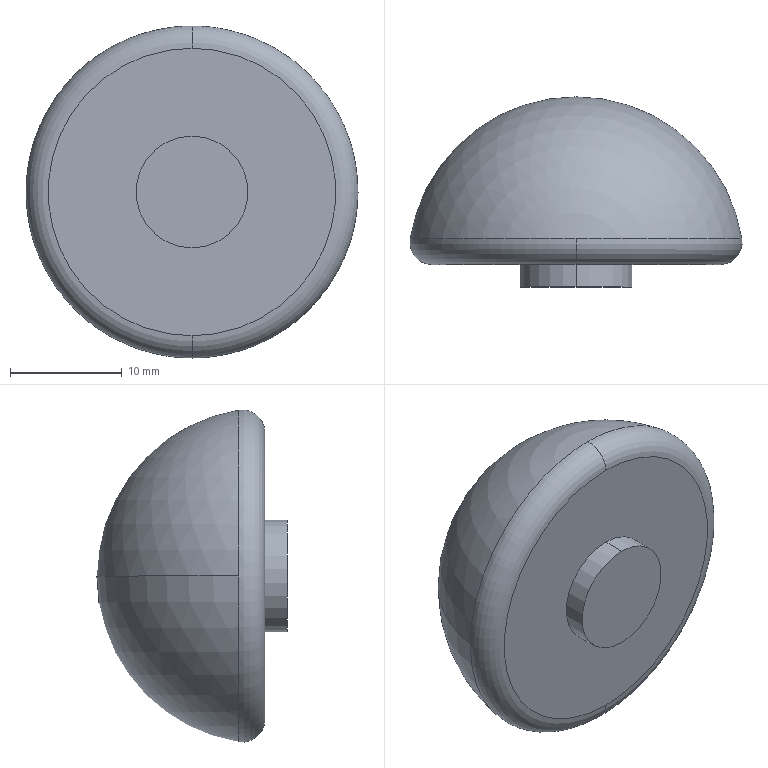Part | SolidWorks | features Fillet 1, ICE 1, Revolution 1 | 1 solid | 8 faces | box 29.69 x 17 x 29.69 mm | volume 7127 mm3 | torus 2 | cylinder 2 | sphere 2 | plane 2 | commonest cylinder face diameters 10 x2
STEP:
#1=CARTESIAN_POINT('',(0.,2.308,14.821));
#2=VERTEX_POINT('',#1);
#3=CARTESIAN_POINT('',(14.821,2.308,0.));
#4=VERTEX_POINT('',#3);
#5=CARTESIAN_POINT('',(0.,2.308,0.));
#6=DIRECTION('',(0.,1.,0.));
#7=DIRECTION('',(0.,0.,-1.));
#8=AXIS2_PLACEMENT_3D('',#5,#6,#7);
#9=CIRCLE('',#8,14.821);
#10=EDGE_CURVE('',#2,#4,#9,.T.);
#11=ORIENTED_EDGE('',*,*,#10,.F.);
#12=CARTESIAN_POINT('',(0.,0.,12.845));
#13=VERTEX_POINT('',#12);
#14=CARTESIAN_POINT('',(0.,2.,12.845));
#15=DIRECTION('',(1.,0.,0.));
#16=DIRECTION('',(0.,0.,-1.));
#17=AXIS2_PLACEMENT_3D('',#14,#15,#16);
#18=CIRCLE('',#17,2.);
#19=EDGE_CURVE('',#2,#13,#18,.T.);
#20=ORIENTED_EDGE('',*,*,#19,.T.);
#21=CARTESIAN_POINT('',(0.,0.,-12.845));
#22=VERTEX_POINT('',#21);
#23=CARTESIAN_POINT('',(0.,0.,0.));
#24=DIRECTION('',(0.,-1.,0.));
#25=DIRECTION('',(0.,0.,-1.));
#26=AXIS2_PLACEMENT_3D('',#23,#24,#25);
#27=CIRCLE('',#26,12.845);
#28=EDGE_CURVE('',#22,#13,#27,.T.);
#29=ORIENTED_EDGE('',*,*,#28,.F.);
#30=CARTESIAN_POINT('',(0.,2.308,-14.821));
#31=VERTEX_POINT('',#30);
#32=CARTESIAN_POINT('',(0.,2.,-12.845));
#33=DIRECTION('',(-1.,0.,0.));
#34=DIRECTION('',(0.,0.,1.));
#35=AXIS2_PLACEMENT_3D('',#32,#33,#34);
#36=CIRCLE('',#35,2.);
#37=EDGE_CURVE('',#31,#22,#36,.T.);
#38=ORIENTED_EDGE('',*,*,#37,.F.);
#39=CARTESIAN_POINT('',(0.,2.308,0.));
#40=DIRECTION('',(0.,1.,0.));
#41=DIRECTION('',(0.,0.,-1.));
#42=AXIS2_PLACEMENT_3D('',#39,#40,#41);
#43=CIRCLE('',#42,14.821);
#44=EDGE_CURVE('',#4,#31,#43,.T.);
#45=ORIENTED_EDGE('',*,*,#44,.F.);
#46=EDGE_LOOP('',(#11,#20,#29,#38,#45));
#47=FACE_OUTER_BOUND('',#46,.T.);
#48=CARTESIAN_POINT('',(0.,2.,0.));
#49=DIRECTION('',(0.,-1.,0.));
#50=DIRECTION('',(0.,0.,-1.));
#51=AXIS2_PLACEMENT_3D('',#48,#49,#50);
#52=TOROIDAL_SURFACE('',#51,12.845,2.);
#53=ADVANCED_FACE('',(#47),#52,.T.);
#54=CARTESIAN_POINT('',(0.,-2.,-5.));
#55=VERTEX_POINT('',#54);
#56=CARTESIAN_POINT('',(0.,-2.,5.));
#57=VERTEX_POINT('',#56);
#58=CARTESIAN_POINT('',(0.,-2.,0.));
#59=DIRECTION('',(0.,-1.,0.));
#60=DIRECTION('',(0.,0.,-1.));
#61=AXIS2_PLACEMENT_3D('',#58,#59,#60);
#62=CIRCLE('',#61,5.);
#63=EDGE_CURVE('',#55,#57,#62,.T.);
#64=ORIENTED_EDGE('',*,*,#63,.F.);
#65=CARTESIAN_POINT('',(0.,0.,-5.));
#66=VERTEX_POINT('',#65);
#67=CARTESIAN_POINT('',(0.,-2.,-5.));
#68=DIRECTION('',(0.,1.,0.));
#69=VECTOR('',#68,1000.);
#70=LINE('',#67,#69);
#71=EDGE_CURVE('',#55,#66,#70,.T.);
#72=ORIENTED_EDGE('',*,*,#71,.T.);
#73=CARTESIAN_POINT('',(0.,0.,5.));
#74=VERTEX_POINT('',#73);
#75=CARTESIAN_POINT('',(0.,0.,0.));
#76=DIRECTION('',(0.,-1.,0.));
#77=DIRECTION('',(0.,0.,-1.));
#78=AXIS2_PLACEMENT_3D('',#75,#76,#77);
#79=CIRCLE('',#78,5.);
#80=EDGE_CURVE('',#66,#74,#79,.T.);
#81=ORIENTED_EDGE('',*,*,#80,.T.);
#82=CARTESIAN_POINT('',(0.,-2.,5.));
#83=DIRECTION('',(0.,1.,0.));
#84=VECTOR('',#83,1000.);
#85=LINE('',#82,#84);
#86=EDGE_CURVE('',#57,#74,#85,.T.);
#87=ORIENTED_EDGE('',*,*,#86,.F.);
#88=EDGE_LOOP('',(#64,#72,#81,#87));
#89=FACE_OUTER_BOUND('',#88,.T.);
#90=CARTESIAN_POINT('',(0.,-2.,0.));
#91=DIRECTION('',(0.,1.,0.));
#92=DIRECTION('',(0.,0.,1.));
#93=AXIS2_PLACEMENT_3D('',#90,#91,#92);
#94=CYLINDRICAL_SURFACE('',#93,5.);
#95=ADVANCED_FACE('',(#89),#94,.T.);
#96=CARTESIAN_POINT('',(0.,15.,0.));
#97=VERTEX_POINT('',#96);
#98=CARTESIAN_POINT('',(0.,0.,0.));
#99=DIRECTION('',(0.,0.,-1.));
#100=DIRECTION('',(-1.,0.,0.));
#101=AXIS2_PLACEMENT_3D('',#98,#99,#100);
#102=CIRCLE('',#101,15.);
#103=EDGE_CURVE('',#97,#4,#102,.T.);
#104=ORIENTED_EDGE('',*,*,#103,.F.);
#105=CARTESIAN_POINT('',(-14.821,2.308,0.));
#106=VERTEX_POINT('',#105);
#107=CARTESIAN_POINT('',(0.,0.,0.));
#108=DIRECTION('',(0.,0.,1.));
#109=DIRECTION('',(1.,0.,0.));
#110=AXIS2_PLACEMENT_3D('',#107,#108,#109);
#111=CIRCLE('',#110,15.);
#112=EDGE_CURVE('',#97,#106,#111,.T.);
#113=ORIENTED_EDGE('',*,*,#112,.T.);
#114=CARTESIAN_POINT('',(0.,2.308,0.));
#115=DIRECTION('',(0.,1.,0.));
#116=DIRECTION('',(0.,0.,-1.));
#117=AXIS2_PLACEMENT_3D('',#114,#115,#116);
#118=CIRCLE('',#117,14.821);
#119=EDGE_CURVE('',#106,#2,#118,.T.);
#120=ORIENTED_EDGE('',*,*,#119,.T.);
#121=ORIENTED_EDGE('',*,*,#10,.T.);
#122=EDGE_LOOP('',(#104,#113,#120,#121));
#123=FACE_OUTER_BOUND('',#122,.T.);
#124=CARTESIAN_POINT('',(0.,0.,0.));
#125=DIRECTION('',(0.,0.,1.));
#126=DIRECTION('',(1.,0.,0.));
#127=AXIS2_PLACEMENT_3D('',#124,#125,#126);
#128=SPHERICAL_SURFACE('',#127,15.);
#129=ADVANCED_FACE('',(#123),#128,.T.);
#130=ORIENTED_EDGE('',*,*,#28,.T.);
#131=CARTESIAN_POINT('',(0.,0.,0.));
#132=DIRECTION('',(0.,-1.,0.));
#133=DIRECTION('',(0.,0.,-1.));
#134=AXIS2_PLACEMENT_3D('',#131,#132,#133);
#135=CIRCLE('',#134,12.845);
#136=EDGE_CURVE('',#13,#22,#135,.T.);
#137=ORIENTED_EDGE('',*,*,#136,.T.);
#138=EDGE_LOOP('',(#130,#137));
#139=FACE_OUTER_BOUND('',#138,.T.);
#140=CARTESIAN_POINT('',(0.,0.,0.));
#141=DIRECTION('',(0.,-1.,0.));
#142=DIRECTION('',(0.,0.,-1.));
#143=AXIS2_PLACEMENT_3D('',#140,#141,#142);
#144=CIRCLE('',#143,5.);
#145=EDGE_CURVE('',#74,#66,#144,.T.);
#146=ORIENTED_EDGE('',*,*,#145,.F.);
#147=ORIENTED_EDGE('',*,*,#80,.F.);
#148=EDGE_LOOP('',(#146,#147));
#149=FACE_BOUND('',#148,.T.);
#150=CARTESIAN_POINT('',(0.,0.,0.));
#151=DIRECTION('',(0.,-1.,0.));
#152=DIRECTION('',(0.,0.,-1.));
#153=AXIS2_PLACEMENT_3D('',#150,#151,#152);
#154=PLANE('',#153);
#155=ADVANCED_FACE('',(#139,#149),#154,.T.);
#156=ORIENTED_EDGE('',*,*,#112,.F.);
#157=ORIENTED_EDGE('',*,*,#103,.T.);
#158=ORIENTED_EDGE('',*,*,#44,.T.);
#159=CARTESIAN_POINT('',(0.,2.308,0.));
#160=DIRECTION('',(0.,1.,0.));
#161=DIRECTION('',(0.,0.,-1.));
#162=AXIS2_PLACEMENT_3D('',#159,#160,#161);
#163=CIRCLE('',#162,14.821);
#164=EDGE_CURVE('',#31,#106,#163,.T.);
#165=ORIENTED_EDGE('',*,*,#164,.T.);
#166=EDGE_LOOP('',(#156,#157,#158,#165));
#167=FACE_OUTER_BOUND('',#166,.T.);
#168=CARTESIAN_POINT('',(0.,0.,0.));
#169=DIRECTION('',(0.,0.,1.));
#170=DIRECTION('',(1.,0.,0.));
#171=AXIS2_PLACEMENT_3D('',#168,#169,#170);
#172=SPHERICAL_SURFACE('',#171,15.);
#173=ADVANCED_FACE('',(#167),#172,.T.);
#174=ORIENTED_EDGE('',*,*,#71,.F.);
#175=CARTESIAN_POINT('',(0.,-2.,0.));
#176=DIRECTION('',(0.,-1.,0.));
#177=DIRECTION('',(0.,0.,-1.));
#178=AXIS2_PLACEMENT_3D('',#175,#176,#177);
#179=CIRCLE('',#178,5.);
#180=EDGE_CURVE('',#57,#55,#179,.T.);
#181=ORIENTED_EDGE('',*,*,#180,.F.);
#182=ORIENTED_EDGE('',*,*,#86,.T.);
#183=ORIENTED_EDGE('',*,*,#145,.T.);
#184=EDGE_LOOP('',(#174,#181,#182,#183));
#185=FACE_OUTER_BOUND('',#184,.T.);
#186=CARTESIAN_POINT('',(0.,-2.,0.));
#187=DIRECTION('',(0.,1.,0.));
#188=DIRECTION('',(0.,0.,1.));
#189=AXIS2_PLACEMENT_3D('',#186,#187,#188);
#190=CYLINDRICAL_SURFACE('',#189,5.);
#191=ADVANCED_FACE('',(#185),#190,.T.);
#192=ORIENTED_EDGE('',*,*,#180,.T.);
#193=ORIENTED_EDGE('',*,*,#63,.T.);
#194=EDGE_LOOP('',(#192,#193));
#195=FACE_OUTER_BOUND('',#194,.T.);
#196=CARTESIAN_POINT('',(0.,-2.,0.));
#197=DIRECTION('',(0.,-1.,0.));
#198=DIRECTION('',(0.,0.,-1.));
#199=AXIS2_PLACEMENT_3D('',#196,#197,#198);
#200=PLANE('',#199);
#201=ADVANCED_FACE('',(#195),#200,.T.);
#202=ORIENTED_EDGE('',*,*,#19,.F.);
#203=ORIENTED_EDGE('',*,*,#119,.F.);
#204=ORIENTED_EDGE('',*,*,#164,.F.);
#205=ORIENTED_EDGE('',*,*,#37,.T.);
#206=ORIENTED_EDGE('',*,*,#136,.F.);
#207=EDGE_LOOP('',(#202,#203,#204,#205,#206));
#208=FACE_OUTER_BOUND('',#207,.T.);
#209=CARTESIAN_POINT('',(0.,2.,0.));
#210=DIRECTION('',(0.,-1.,0.));
#211=DIRECTION('',(0.,0.,-1.));
#212=AXIS2_PLACEMENT_3D('',#209,#210,#211);
#213=TOROIDAL_SURFACE('',#212,12.845,2.);
#214=ADVANCED_FACE('',(#208),#213,.T.);
#215=CLOSED_SHELL('',(#53,#95,#129,#155,#173,#191,#201,#214));
#216=MANIFOLD_SOLID_BREP('',#215);
#217=CARTESIAN_POINT('',(0.,0.,0.));
#218=DIRECTION('',(0.,0.,1.));
#219=DIRECTION('',(1.,0.,0.));
#220=AXIS2_PLACEMENT_3D('',#217,#218,#219);
#221=(LENGTH_UNIT()NAMED_UNIT(*)SI_UNIT(.MILLI.,.METRE.));
#222=UNCERTAINTY_MEASURE_WITH_UNIT(LENGTH_MEASURE(0.00001),#221,'','');
#223=(NAMED_UNIT(*)PLANE_ANGLE_UNIT()SI_UNIT($,.RADIAN.));
#224=(NAMED_UNIT(*)SI_UNIT($,.STERADIAN.)SOLID_ANGLE_UNIT());
#225=(GEOMETRIC_REPRESENTATION_CONTEXT(3)GLOBAL_UNCERTAINTY_ASSIGNED_CONTEXT((#222))GLOBAL_UNIT_ASSIGNED_CONTEXT((#221,#223,#224))REPRESENTATION_CONTEXT('',''));
#226=ADVANCED_BREP_SHAPE_REPRESENTATION('',(#216,#220),#225);